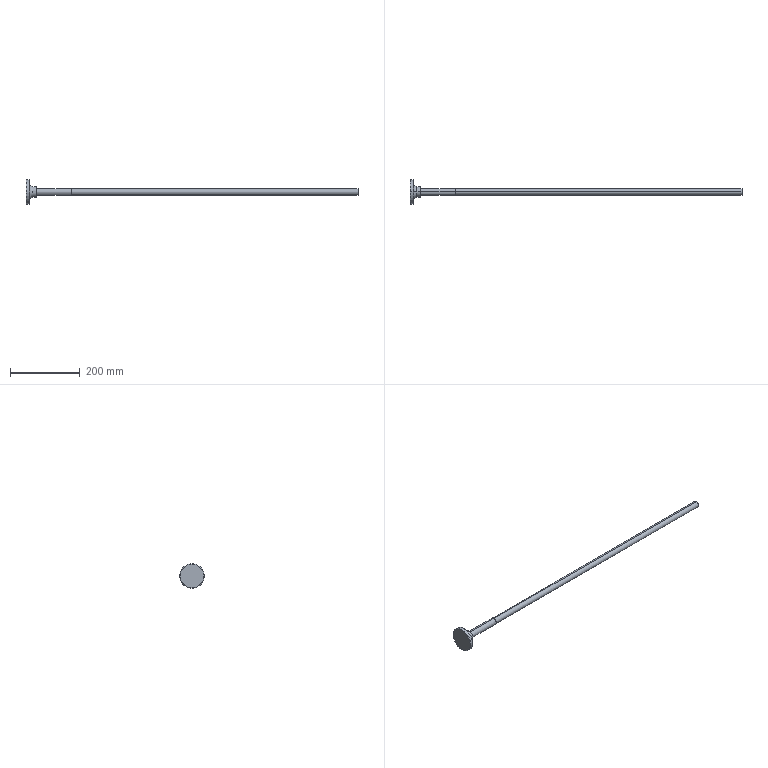Part | SolidWorks | features ICE 3, Chamfer 1, Extrusion 1, Fillet 1 | 1 solid | 19 faces | box 950 x 70 x 70 mm | volume 294808 mm3 | cylinder 8 | plane 5 | cone 4 | torus 2 | commonest cylinder face diameters 18 x2 20 x2 30 x2 70 x2
STEP:
#1=CARTESIAN_POINT('',(20.,0.,15.));
#2=VERTEX_POINT('',#1);
#3=CARTESIAN_POINT('',(20.,0.,-15.));
#4=VERTEX_POINT('',#3);
#5=CARTESIAN_POINT('',(20.,0.,0.));
#6=DIRECTION('',(1.,0.,0.));
#7=DIRECTION('',(0.,0.,-1.));
#8=AXIS2_PLACEMENT_3D('',#5,#6,#7);
#9=CIRCLE('',#8,15.);
#10=EDGE_CURVE('',#2,#4,#9,.T.);
#11=ORIENTED_EDGE('',*,*,#10,.F.);
#12=CARTESIAN_POINT('',(10.,0.,25.));
#13=VERTEX_POINT('',#12);
#14=CARTESIAN_POINT('',(20.,0.,25.));
#15=DIRECTION('',(0.,1.,0.));
#16=DIRECTION('',(0.,0.,1.));
#17=AXIS2_PLACEMENT_3D('',#14,#15,#16);
#18=CIRCLE('',#17,10.);
#19=EDGE_CURVE('',#2,#13,#18,.T.);
#20=ORIENTED_EDGE('',*,*,#19,.T.);
#21=CARTESIAN_POINT('',(10.,0.,-25.));
#22=VERTEX_POINT('',#21);
#23=CARTESIAN_POINT('',(10.,0.,0.));
#24=DIRECTION('',(-1.,0.,0.));
#25=DIRECTION('',(0.,0.,-1.));
#26=AXIS2_PLACEMENT_3D('',#23,#24,#25);
#27=CIRCLE('',#26,25.);
#28=EDGE_CURVE('',#22,#13,#27,.T.);
#29=ORIENTED_EDGE('',*,*,#28,.F.);
#30=CARTESIAN_POINT('',(20.,0.,-25.));
#31=DIRECTION('',(0.,-1.,0.));
#32=DIRECTION('',(0.,0.,-1.));
#33=AXIS2_PLACEMENT_3D('',#30,#31,#32);
#34=CIRCLE('',#33,10.);
#35=EDGE_CURVE('',#4,#22,#34,.T.);
#36=ORIENTED_EDGE('',*,*,#35,.F.);
#37=EDGE_LOOP('',(#11,#20,#29,#36));
#38=FACE_OUTER_BOUND('',#37,.T.);
#39=CARTESIAN_POINT('',(20.,0.,0.));
#40=DIRECTION('',(1.,0.,0.));
#41=DIRECTION('',(0.,0.,-1.));
#42=AXIS2_PLACEMENT_3D('',#39,#40,#41);
#43=TOROIDAL_SURFACE('',#42,25.,10.);
#44=ADVANCED_FACE('',(#38),#43,.F.);
#45=CARTESIAN_POINT('',(10.,0.,-34.));
#46=VERTEX_POINT('',#45);
#47=CARTESIAN_POINT('',(10.,0.,34.));
#48=VERTEX_POINT('',#47);
#49=CARTESIAN_POINT('',(10.,0.,0.));
#50=DIRECTION('',(1.,0.,0.));
#51=DIRECTION('',(0.,0.,-1.));
#52=AXIS2_PLACEMENT_3D('',#49,#50,#51);
#53=CIRCLE('',#52,34.);
#54=EDGE_CURVE('',#46,#48,#53,.T.);
#55=ORIENTED_EDGE('',*,*,#54,.F.);
#56=CARTESIAN_POINT('',(9.,0.,-35.));
#57=VERTEX_POINT('',#56);
#58=CARTESIAN_POINT('',(10.,0.,-34.));
#59=DIRECTION('',(-0.7071,0.,-0.7071));
#60=VECTOR('',#59,1000.);
#61=LINE('',#58,#60);
#62=EDGE_CURVE('',#46,#57,#61,.T.);
#63=ORIENTED_EDGE('',*,*,#62,.T.);
#64=CARTESIAN_POINT('',(9.,0.,35.));
#65=VERTEX_POINT('',#64);
#66=CARTESIAN_POINT('',(9.,0.,0.));
#67=DIRECTION('',(-1.,0.,0.));
#68=DIRECTION('',(0.,0.,-1.));
#69=AXIS2_PLACEMENT_3D('',#66,#67,#68);
#70=CIRCLE('',#69,35.);
#71=EDGE_CURVE('',#65,#57,#70,.T.);
#72=ORIENTED_EDGE('',*,*,#71,.F.);
#73=CARTESIAN_POINT('',(10.,0.,34.));
#74=DIRECTION('',(-0.7071,0.,0.7071));
#75=VECTOR('',#74,1000.);
#76=LINE('',#73,#75);
#77=EDGE_CURVE('',#48,#65,#76,.T.);
#78=ORIENTED_EDGE('',*,*,#77,.F.);
#79=EDGE_LOOP('',(#55,#63,#72,#78));
#80=FACE_OUTER_BOUND('',#79,.T.);
#81=CARTESIAN_POINT('',(10.,0.,0.));
#82=DIRECTION('',(-1.,0.,0.));
#83=DIRECTION('',(0.,0.,1.));
#84=AXIS2_PLACEMENT_3D('',#81,#82,#83);
#85=CONICAL_SURFACE('',#84,34.,0.7854);
#86=ADVANCED_FACE('',(#80),#85,.T.);
#87=CARTESIAN_POINT('',(0.,0.,34.));
#88=VERTEX_POINT('',#87);
#89=CARTESIAN_POINT('',(0.,0.,-34.));
#90=VERTEX_POINT('',#89);
#91=CARTESIAN_POINT('',(0.,0.,0.));
#92=DIRECTION('',(-1.,0.,0.));
#93=DIRECTION('',(0.,0.,-1.));
#94=AXIS2_PLACEMENT_3D('',#91,#92,#93);
#95=CIRCLE('',#94,34.);
#96=EDGE_CURVE('',#88,#90,#95,.T.);
#97=ORIENTED_EDGE('',*,*,#96,.F.);
#98=CARTESIAN_POINT('',(1.,0.,35.));
#99=VERTEX_POINT('',#98);
#100=CARTESIAN_POINT('',(1.,0.,35.));
#101=DIRECTION('',(0.7071,0.,0.7071));
#102=VECTOR('',#101,1000.);
#103=LINE('',#100,#102);
#104=EDGE_CURVE('',#88,#99,#103,.T.);
#105=ORIENTED_EDGE('',*,*,#104,.T.);
#106=CARTESIAN_POINT('',(1.,0.,-35.));
#107=VERTEX_POINT('',#106);
#108=CARTESIAN_POINT('',(1.,0.,0.));
#109=DIRECTION('',(1.,0.,0.));
#110=DIRECTION('',(0.,0.,-1.));
#111=AXIS2_PLACEMENT_3D('',#108,#109,#110);
#112=CIRCLE('',#111,35.);
#113=EDGE_CURVE('',#107,#99,#112,.T.);
#114=ORIENTED_EDGE('',*,*,#113,.F.);
#115=CARTESIAN_POINT('',(1.,0.,-35.));
#116=DIRECTION('',(0.7071,0.,-0.7071));
#117=VECTOR('',#116,1000.);
#118=LINE('',#115,#117);
#119=EDGE_CURVE('',#90,#107,#118,.T.);
#120=ORIENTED_EDGE('',*,*,#119,.F.);
#121=EDGE_LOOP('',(#97,#105,#114,#120));
#122=FACE_OUTER_BOUND('',#121,.T.);
#123=CARTESIAN_POINT('',(1.,0.,0.));
#124=DIRECTION('',(1.,0.,0.));
#125=DIRECTION('',(0.,0.,-1.));
#126=AXIS2_PLACEMENT_3D('',#123,#124,#125);
#127=CONICAL_SURFACE('',#126,35.,0.7854);
#128=ADVANCED_FACE('',(#122),#127,.T.);
#129=CARTESIAN_POINT('',(950.,0.,-9.));
#130=VERTEX_POINT('',#129);
#131=CARTESIAN_POINT('',(950.,0.,9.));
#132=VERTEX_POINT('',#131);
#133=CARTESIAN_POINT('',(950.,0.,0.));
#134=DIRECTION('',(1.,0.,0.));
#135=DIRECTION('',(0.,0.,-1.));
#136=AXIS2_PLACEMENT_3D('',#133,#134,#135);
#137=CIRCLE('',#136,9.);
#138=EDGE_CURVE('',#130,#132,#137,.T.);
#139=ORIENTED_EDGE('',*,*,#138,.F.);
#140=CARTESIAN_POINT('',(130.,0.,-9.));
#141=VERTEX_POINT('',#140);
#142=CARTESIAN_POINT('',(950.,0.,-9.));
#143=DIRECTION('',(-1.,0.,0.));
#144=VECTOR('',#143,1000.);
#145=LINE('',#142,#144);
#146=EDGE_CURVE('',#130,#141,#145,.T.);
#147=ORIENTED_EDGE('',*,*,#146,.T.);
#148=CARTESIAN_POINT('',(130.,0.,9.));
#149=VERTEX_POINT('',#148);
#150=CARTESIAN_POINT('',(130.,0.,0.));
#151=DIRECTION('',(1.,0.,0.));
#152=DIRECTION('',(0.,0.,-1.));
#153=AXIS2_PLACEMENT_3D('',#150,#151,#152);
#154=CIRCLE('',#153,9.);
#155=EDGE_CURVE('',#141,#149,#154,.T.);
#156=ORIENTED_EDGE('',*,*,#155,.T.);
#157=CARTESIAN_POINT('',(950.,0.,9.));
#158=DIRECTION('',(-1.,0.,0.));
#159=VECTOR('',#158,1000.);
#160=LINE('',#157,#159);
#161=EDGE_CURVE('',#132,#149,#160,.T.);
#162=ORIENTED_EDGE('',*,*,#161,.F.);
#163=EDGE_LOOP('',(#139,#147,#156,#162));
#164=FACE_OUTER_BOUND('',#163,.T.);
#165=CARTESIAN_POINT('',(950.,0.,0.));
#166=DIRECTION('',(-1.,0.,0.));
#167=DIRECTION('',(0.,0.,1.));
#168=AXIS2_PLACEMENT_3D('',#165,#166,#167);
#169=CYLINDRICAL_SURFACE('',#168,9.);
#170=ADVANCED_FACE('',(#164),#169,.T.);
#171=CARTESIAN_POINT('',(130.,0.,-10.));
#172=VERTEX_POINT('',#171);
#173=CARTESIAN_POINT('',(130.,0.,10.));
#174=VERTEX_POINT('',#173);
#175=CARTESIAN_POINT('',(130.,0.,0.));
#176=DIRECTION('',(1.,0.,0.));
#177=DIRECTION('',(0.,0.,-1.));
#178=AXIS2_PLACEMENT_3D('',#175,#176,#177);
#179=CIRCLE('',#178,10.);
#180=EDGE_CURVE('',#172,#174,#179,.T.);
#181=ORIENTED_EDGE('',*,*,#180,.F.);
#182=CARTESIAN_POINT('',(30.,0.,-10.));
#183=VERTEX_POINT('',#182);
#184=CARTESIAN_POINT('',(130.,0.,-10.));
#185=DIRECTION('',(-1.,0.,0.));
#186=VECTOR('',#185,1000.);
#187=LINE('',#184,#186);
#188=EDGE_CURVE('',#172,#183,#187,.T.);
#189=ORIENTED_EDGE('',*,*,#188,.T.);
#190=CARTESIAN_POINT('',(30.,0.,10.));
#191=VERTEX_POINT('',#190);
#192=CARTESIAN_POINT('',(30.,0.,0.));
#193=DIRECTION('',(1.,0.,0.));
#194=DIRECTION('',(0.,0.,-1.));
#195=AXIS2_PLACEMENT_3D('',#192,#193,#194);
#196=CIRCLE('',#195,10.);
#197=EDGE_CURVE('',#183,#191,#196,.T.);
#198=ORIENTED_EDGE('',*,*,#197,.T.);
#199=CARTESIAN_POINT('',(130.,0.,10.));
#200=DIRECTION('',(-1.,0.,0.));
#201=VECTOR('',#200,1000.);
#202=LINE('',#199,#201);
#203=EDGE_CURVE('',#174,#191,#202,.T.);
#204=ORIENTED_EDGE('',*,*,#203,.F.);
#205=EDGE_LOOP('',(#181,#189,#198,#204));
#206=FACE_OUTER_BOUND('',#205,.T.);
#207=CARTESIAN_POINT('',(130.,0.,0.));
#208=DIRECTION('',(-1.,0.,0.));
#209=DIRECTION('',(0.,0.,1.));
#210=AXIS2_PLACEMENT_3D('',#207,#208,#209);
#211=CYLINDRICAL_SURFACE('',#210,10.);
#212=ADVANCED_FACE('',(#206),#211,.T.);
#213=CARTESIAN_POINT('',(30.,0.,-15.));
#214=VERTEX_POINT('',#213);
#215=CARTESIAN_POINT('',(30.,0.,15.));
#216=VERTEX_POINT('',#215);
#217=CARTESIAN_POINT('',(30.,0.,0.));
#218=DIRECTION('',(1.,0.,0.));
#219=DIRECTION('',(0.,0.,-1.));
#220=AXIS2_PLACEMENT_3D('',#217,#218,#219);
#221=CIRCLE('',#220,15.);
#222=EDGE_CURVE('',#214,#216,#221,.T.);
#223=ORIENTED_EDGE('',*,*,#222,.F.);
#224=CARTESIAN_POINT('',(30.,0.,-15.));
#225=DIRECTION('',(-1.,0.,0.));
#226=VECTOR('',#225,1000.);
#227=LINE('',#224,#226);
#228=EDGE_CURVE('',#214,#4,#227,.T.);
#229=ORIENTED_EDGE('',*,*,#228,.T.);
#230=CARTESIAN_POINT('',(20.,0.,0.));
#231=DIRECTION('',(1.,0.,0.));
#232=DIRECTION('',(0.,0.,-1.));
#233=AXIS2_PLACEMENT_3D('',#230,#231,#232);
#234=CIRCLE('',#233,15.);
#235=EDGE_CURVE('',#4,#2,#234,.T.);
#236=ORIENTED_EDGE('',*,*,#235,.T.);
#237=CARTESIAN_POINT('',(30.,0.,15.));
#238=DIRECTION('',(-1.,0.,0.));
#239=VECTOR('',#238,1000.);
#240=LINE('',#237,#239);
#241=EDGE_CURVE('',#216,#2,#240,.T.);
#242=ORIENTED_EDGE('',*,*,#241,.F.);
#243=EDGE_LOOP('',(#223,#229,#236,#242));
#244=FACE_OUTER_BOUND('',#243,.T.);
#245=CARTESIAN_POINT('',(30.,0.,0.));
#246=DIRECTION('',(-1.,0.,0.));
#247=DIRECTION('',(0.,0.,1.));
#248=AXIS2_PLACEMENT_3D('',#245,#246,#247);
#249=CYLINDRICAL_SURFACE('',#248,15.);
#250=ADVANCED_FACE('',(#244),#249,.T.);
#251=ORIENTED_EDGE('',*,*,#71,.T.);
#252=CARTESIAN_POINT('',(10.,0.,-35.));
#253=DIRECTION('',(-1.,0.,0.));
#254=VECTOR('',#253,1000.);
#255=LINE('',#252,#254);
#256=EDGE_CURVE('',#57,#107,#255,.T.);
#257=ORIENTED_EDGE('',*,*,#256,.T.);
#258=ORIENTED_EDGE('',*,*,#113,.T.);
#259=CARTESIAN_POINT('',(10.,0.,35.));
#260=DIRECTION('',(-1.,0.,0.));
#261=VECTOR('',#260,1000.);
#262=LINE('',#259,#261);
#263=EDGE_CURVE('',#65,#99,#262,.T.);
#264=ORIENTED_EDGE('',*,*,#263,.F.);
#265=EDGE_LOOP('',(#251,#257,#258,#264));
#266=FACE_OUTER_BOUND('',#265,.T.);
#267=CARTESIAN_POINT('',(10.,0.,0.));
#268=DIRECTION('',(-1.,0.,0.));
#269=DIRECTION('',(0.,0.,1.));
#270=AXIS2_PLACEMENT_3D('',#267,#268,#269);
#271=CYLINDRICAL_SURFACE('',#270,35.);
#272=ADVANCED_FACE('',(#266),#271,.T.);
#273=ORIENTED_EDGE('',*,*,#256,.F.);
#274=CARTESIAN_POINT('',(9.,0.,0.));
#275=DIRECTION('',(-1.,0.,0.));
#276=DIRECTION('',(0.,0.,-1.));
#277=AXIS2_PLACEMENT_3D('',#274,#275,#276);
#278=CIRCLE('',#277,35.);
#279=EDGE_CURVE('',#57,#65,#278,.T.);
#280=ORIENTED_EDGE('',*,*,#279,.T.);
#281=ORIENTED_EDGE('',*,*,#263,.T.);
#282=CARTESIAN_POINT('',(1.,0.,0.));
#283=DIRECTION('',(1.,0.,0.));
#284=DIRECTION('',(0.,0.,-1.));
#285=AXIS2_PLACEMENT_3D('',#282,#283,#284);
#286=CIRCLE('',#285,35.);
#287=EDGE_CURVE('',#99,#107,#286,.T.);
#288=ORIENTED_EDGE('',*,*,#287,.T.);
#289=EDGE_LOOP('',(#273,#280,#281,#288));
#290=FACE_OUTER_BOUND('',#289,.T.);
#291=CARTESIAN_POINT('',(10.,0.,0.));
#292=DIRECTION('',(-1.,0.,0.));
#293=DIRECTION('',(0.,0.,1.));
#294=AXIS2_PLACEMENT_3D('',#291,#292,#293);
#295=CYLINDRICAL_SURFACE('',#294,35.);
#296=ADVANCED_FACE('',(#290),#295,.T.);
#297=ORIENTED_EDGE('',*,*,#28,.T.);
#298=CARTESIAN_POINT('',(10.,0.,0.));
#299=DIRECTION('',(-1.,0.,0.));
#300=DIRECTION('',(0.,0.,-1.));
#301=AXIS2_PLACEMENT_3D('',#298,#299,#300);
#302=CIRCLE('',#301,25.);
#303=EDGE_CURVE('',#13,#22,#302,.T.);
#304=ORIENTED_EDGE('',*,*,#303,.T.);
#305=EDGE_LOOP('',(#297,#304));
#306=FACE_BOUND('',#305,.T.);
#307=CARTESIAN_POINT('',(10.,0.,0.));
#308=DIRECTION('',(1.,0.,0.));
#309=DIRECTION('',(0.,0.,-1.));
#310=AXIS2_PLACEMENT_3D('',#307,#308,#309);
#311=CIRCLE('',#310,34.);
#312=EDGE_CURVE('',#48,#46,#311,.T.);
#313=ORIENTED_EDGE('',*,*,#312,.T.);
#314=ORIENTED_EDGE('',*,*,#54,.T.);
#315=EDGE_LOOP('',(#313,#314));
#316=FACE_OUTER_BOUND('',#315,.T.);
#317=CARTESIAN_POINT('',(10.,0.,0.));
#318=DIRECTION('',(1.,0.,0.));
#319=DIRECTION('',(0.,0.,-1.));
#320=AXIS2_PLACEMENT_3D('',#317,#318,#319);
#321=PLANE('',#320);
#322=ADVANCED_FACE('',(#306,#316),#321,.T.);
#323=CARTESIAN_POINT('',(0.,0.,0.));
#324=DIRECTION('',(-1.,0.,0.));
#325=DIRECTION('',(0.,0.,-1.));
#326=AXIS2_PLACEMENT_3D('',#323,#324,#325);
#327=CIRCLE('',#326,34.);
#328=EDGE_CURVE('',#90,#88,#327,.T.);
#329=ORIENTED_EDGE('',*,*,#328,.T.);
#330=ORIENTED_EDGE('',*,*,#96,.T.);
#331=EDGE_LOOP('',(#329,#330));
#332=FACE_OUTER_BOUND('',#331,.T.);
#333=CARTESIAN_POINT('',(0.,0.,0.));
#334=DIRECTION('',(1.,0.,0.));
#335=DIRECTION('',(0.,0.,-1.));
#336=AXIS2_PLACEMENT_3D('',#333,#334,#335);
#337=PLANE('',#336);
#338=ADVANCED_FACE('',(#332),#337,.F.);
#339=ORIENTED_EDGE('',*,*,#228,.F.);
#340=CARTESIAN_POINT('',(30.,0.,0.));
#341=DIRECTION('',(1.,0.,0.));
#342=DIRECTION('',(0.,0.,-1.));
#343=AXIS2_PLACEMENT_3D('',#340,#341,#342);
#344=CIRCLE('',#343,15.);
#345=EDGE_CURVE('',#216,#214,#344,.T.);
#346=ORIENTED_EDGE('',*,*,#345,.F.);
#347=ORIENTED_EDGE('',*,*,#241,.T.);
#348=ORIENTED_EDGE('',*,*,#10,.T.);
#349=EDGE_LOOP('',(#339,#346,#347,#348));
#350=FACE_OUTER_BOUND('',#349,.T.);
#351=CARTESIAN_POINT('',(30.,0.,0.));
#352=DIRECTION('',(-1.,0.,0.));
#353=DIRECTION('',(0.,0.,1.));
#354=AXIS2_PLACEMENT_3D('',#351,#352,#353);
#355=CYLINDRICAL_SURFACE('',#354,15.);
#356=ADVANCED_FACE('',(#350),#355,.T.);
#357=CARTESIAN_POINT('',(30.,0.,0.));
#358=DIRECTION('',(1.,0.,0.));
#359=DIRECTION('',(0.,0.,-1.));
#360=AXIS2_PLACEMENT_3D('',#357,#358,#359);
#361=CIRCLE('',#360,10.);
#362=EDGE_CURVE('',#191,#183,#361,.T.);
#363=ORIENTED_EDGE('',*,*,#362,.F.);
#364=ORIENTED_EDGE('',*,*,#197,.F.);
#365=EDGE_LOOP('',(#363,#364));
#366=FACE_BOUND('',#365,.T.);
#367=ORIENTED_EDGE('',*,*,#345,.T.);
#368=ORIENTED_EDGE('',*,*,#222,.T.);
#369=EDGE_LOOP('',(#367,#368));
#370=FACE_OUTER_BOUND('',#369,.T.);
#371=CARTESIAN_POINT('',(30.,0.,0.));
#372=DIRECTION('',(1.,0.,0.));
#373=DIRECTION('',(0.,0.,-1.));
#374=AXIS2_PLACEMENT_3D('',#371,#372,#373);
#375=PLANE('',#374);
#376=ADVANCED_FACE('',(#366,#370),#375,.T.);
#377=ORIENTED_EDGE('',*,*,#188,.F.);
#378=CARTESIAN_POINT('',(130.,0.,0.));
#379=DIRECTION('',(1.,0.,0.));
#380=DIRECTION('',(0.,0.,-1.));
#381=AXIS2_PLACEMENT_3D('',#378,#379,#380);
#382=CIRCLE('',#381,10.);
#383=EDGE_CURVE('',#174,#172,#382,.T.);
#384=ORIENTED_EDGE('',*,*,#383,.F.);
#385=ORIENTED_EDGE('',*,*,#203,.T.);
#386=ORIENTED_EDGE('',*,*,#362,.T.);
#387=EDGE_LOOP('',(#377,#384,#385,#386));
#388=FACE_OUTER_BOUND('',#387,.T.);
#389=CARTESIAN_POINT('',(130.,0.,0.));
#390=DIRECTION('',(-1.,0.,0.));
#391=DIRECTION('',(0.,0.,1.));
#392=AXIS2_PLACEMENT_3D('',#389,#390,#391);
#393=CYLINDRICAL_SURFACE('',#392,10.);
#394=ADVANCED_FACE('',(#388),#393,.T.);
#395=CARTESIAN_POINT('',(130.,0.,0.));
#396=DIRECTION('',(1.,0.,0.));
#397=DIRECTION('',(0.,0.,-1.));
#398=AXIS2_PLACEMENT_3D('',#395,#396,#397);
#399=CIRCLE('',#398,9.);
#400=EDGE_CURVE('',#149,#141,#399,.T.);
#401=ORIENTED_EDGE('',*,*,#400,.F.);
#402=ORIENTED_EDGE('',*,*,#155,.F.);
#403=EDGE_LOOP('',(#401,#402));
#404=FACE_BOUND('',#403,.T.);
#405=ORIENTED_EDGE('',*,*,#383,.T.);
#406=ORIENTED_EDGE('',*,*,#180,.T.);
#407=EDGE_LOOP('',(#405,#406));
#408=FACE_OUTER_BOUND('',#407,.T.);
#409=CARTESIAN_POINT('',(130.,0.,0.));
#410=DIRECTION('',(1.,0.,0.));
#411=DIRECTION('',(0.,0.,-1.));
#412=AXIS2_PLACEMENT_3D('',#409,#410,#411);
#413=PLANE('',#412);
#414=ADVANCED_FACE('',(#404,#408),#413,.T.);
#415=ORIENTED_EDGE('',*,*,#146,.F.);
#416=CARTESIAN_POINT('',(950.,0.,0.));
#417=DIRECTION('',(1.,0.,0.));
#418=DIRECTION('',(0.,0.,-1.));
#419=AXIS2_PLACEMENT_3D('',#416,#417,#418);
#420=CIRCLE('',#419,9.);
#421=EDGE_CURVE('',#132,#130,#420,.T.);
#422=ORIENTED_EDGE('',*,*,#421,.F.);
#423=ORIENTED_EDGE('',*,*,#161,.T.);
#424=ORIENTED_EDGE('',*,*,#400,.T.);
#425=EDGE_LOOP('',(#415,#422,#423,#424));
#426=FACE_OUTER_BOUND('',#425,.T.);
#427=CARTESIAN_POINT('',(950.,0.,0.));
#428=DIRECTION('',(-1.,0.,0.));
#429=DIRECTION('',(0.,0.,1.));
#430=AXIS2_PLACEMENT_3D('',#427,#428,#429);
#431=CYLINDRICAL_SURFACE('',#430,9.);
#432=ADVANCED_FACE('',(#426),#431,.T.);
#433=ORIENTED_EDGE('',*,*,#421,.T.);
#434=ORIENTED_EDGE('',*,*,#138,.T.);
#435=EDGE_LOOP('',(#433,#434));
#436=FACE_OUTER_BOUND('',#435,.T.);
#437=CARTESIAN_POINT('',(950.,0.,0.));
#438=DIRECTION('',(1.,0.,0.));
#439=DIRECTION('',(0.,0.,-1.));
#440=AXIS2_PLACEMENT_3D('',#437,#438,#439);
#441=PLANE('',#440);
#442=ADVANCED_FACE('',(#436),#441,.T.);
#443=ORIENTED_EDGE('',*,*,#104,.F.);
#444=ORIENTED_EDGE('',*,*,#328,.F.);
#445=ORIENTED_EDGE('',*,*,#119,.T.);
#446=ORIENTED_EDGE('',*,*,#287,.F.);
#447=EDGE_LOOP('',(#443,#444,#445,#446));
#448=FACE_OUTER_BOUND('',#447,.T.);
#449=CARTESIAN_POINT('',(1.,0.,0.));
#450=DIRECTION('',(1.,0.,0.));
#451=DIRECTION('',(0.,0.,-1.));
#452=AXIS2_PLACEMENT_3D('',#449,#450,#451);
#453=CONICAL_SURFACE('',#452,35.,0.7854);
#454=ADVANCED_FACE('',(#448),#453,.T.);
#455=ORIENTED_EDGE('',*,*,#62,.F.);
#456=ORIENTED_EDGE('',*,*,#312,.F.);
#457=ORIENTED_EDGE('',*,*,#77,.T.);
#458=ORIENTED_EDGE('',*,*,#279,.F.);
#459=EDGE_LOOP('',(#455,#456,#457,#458));
#460=FACE_OUTER_BOUND('',#459,.T.);
#461=CARTESIAN_POINT('',(10.,0.,0.));
#462=DIRECTION('',(-1.,0.,0.));
#463=DIRECTION('',(0.,0.,1.));
#464=AXIS2_PLACEMENT_3D('',#461,#462,#463);
#465=CONICAL_SURFACE('',#464,34.,0.7854);
#466=ADVANCED_FACE('',(#460),#465,.T.);
#467=ORIENTED_EDGE('',*,*,#19,.F.);
#468=ORIENTED_EDGE('',*,*,#235,.F.);
#469=ORIENTED_EDGE('',*,*,#35,.T.);
#470=ORIENTED_EDGE('',*,*,#303,.F.);
#471=EDGE_LOOP('',(#467,#468,#469,#470));
#472=FACE_OUTER_BOUND('',#471,.T.);
#473=CARTESIAN_POINT('',(20.,0.,0.));
#474=DIRECTION('',(1.,0.,0.));
#475=DIRECTION('',(0.,0.,-1.));
#476=AXIS2_PLACEMENT_3D('',#473,#474,#475);
#477=TOROIDAL_SURFACE('',#476,25.,10.);
#478=ADVANCED_FACE('',(#472),#477,.F.);
#479=CLOSED_SHELL('',(#44,#86,#128,#170,#212,#250,#272,#296,#322,#338,#356,#376,#394,#414,#432,#442,#454,#466,#478));
#480=MANIFOLD_SOLID_BREP('',#479);
#481=CARTESIAN_POINT('',(0.,0.,0.));
#482=DIRECTION('',(0.,0.,1.));
#483=DIRECTION('',(1.,0.,0.));
#484=AXIS2_PLACEMENT_3D('',#481,#482,#483);
#485=(LENGTH_UNIT()NAMED_UNIT(*)SI_UNIT(.MILLI.,.METRE.));
#486=UNCERTAINTY_MEASURE_WITH_UNIT(LENGTH_MEASURE(0.00001),#485,'','');
#487=(NAMED_UNIT(*)PLANE_ANGLE_UNIT()SI_UNIT($,.RADIAN.));
#488=(NAMED_UNIT(*)SI_UNIT($,.STERADIAN.)SOLID_ANGLE_UNIT());
#489=(GEOMETRIC_REPRESENTATION_CONTEXT(3)GLOBAL_UNCERTAINTY_ASSIGNED_CONTEXT((#486))GLOBAL_UNIT_ASSIGNED_CONTEXT((#485,#487,#488))REPRESENTATION_CONTEXT('',''));
#490=ADVANCED_BREP_SHAPE_REPRESENTATION('',(#480,#484),#489);